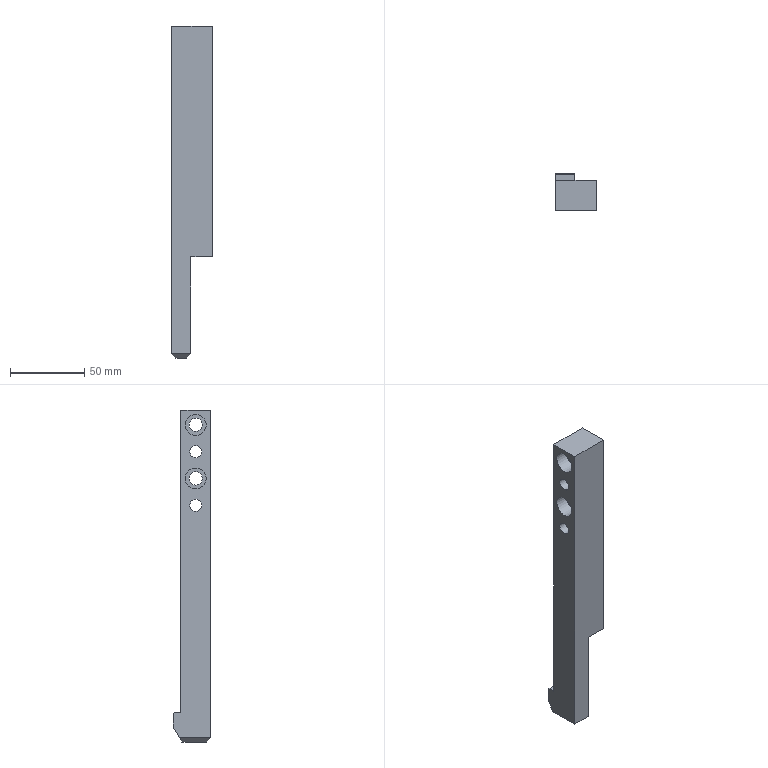Part | STEP file | solid 129 | 1 solid | 23 faces | box 27.5 x 25 x 223 mm | volume 95743 mm3 | plane 17 | cylinder 6 | commonest cylinder face diameters 8 x2 9 x2 14 x2